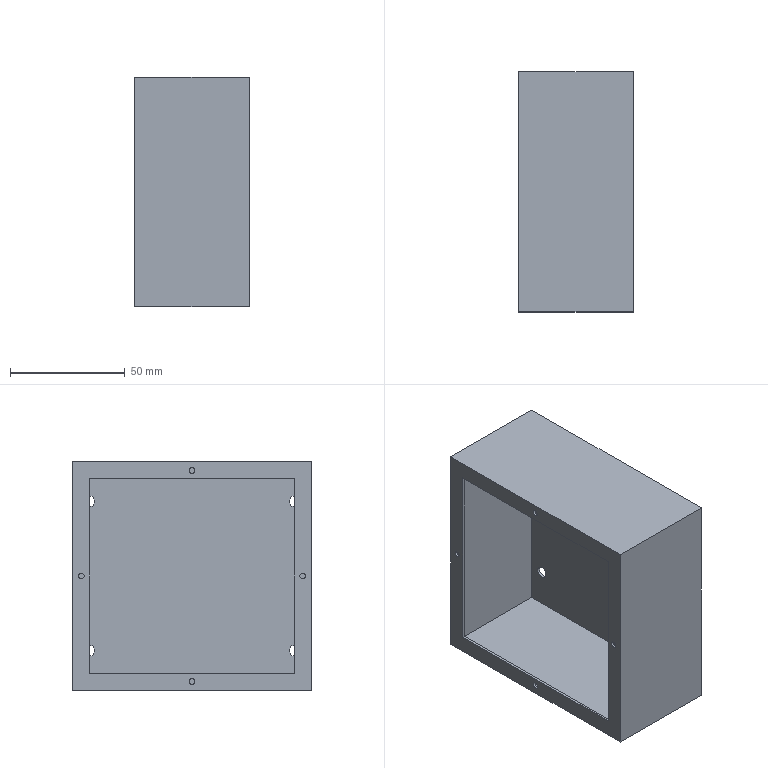Part | STEP file | 2026.6.15-Main Assembly图.sldasm-Part-141 | 1 solid | 32 faces | box 50 x 104.5 x 100 mm | volume 32634 mm3 | cylinder 16 | plane 16 | commonest cylinder face diameters 2.5 x8 5 x8
STEP:
#1=CARTESIAN_POINT('',(-1735.724,608.801,4186.167));
#2=VERTEX_POINT('',#1);
#3=CARTESIAN_POINT('',(-1735.724,606.301,4186.167));
#4=VERTEX_POINT('',#3);
#5=CARTESIAN_POINT('',(-1735.724,607.551,4186.167));
#6=DIRECTION('',(-1.,0.,0.));
#7=DIRECTION('',(0.,0.,1.));
#8=AXIS2_PLACEMENT_3D('',#5,#6,#7);
#9=CIRCLE('',#8,1.25);
#10=EDGE_CURVE('',#2,#4,#9,.T.);
#11=ORIENTED_EDGE('',*,*,#10,.F.);
#12=CARTESIAN_POINT('',(-1736.724,608.801,4186.167));
#13=VERTEX_POINT('',#12);
#14=CARTESIAN_POINT('',(-1735.724,608.801,4186.167));
#15=DIRECTION('',(-1.,0.,0.));
#16=VECTOR('',#15,1000.);
#17=LINE('',#14,#16);
#18=EDGE_CURVE('',#2,#13,#17,.T.);
#19=ORIENTED_EDGE('',*,*,#18,.T.);
#20=CARTESIAN_POINT('',(-1736.724,606.301,4186.167));
#21=VERTEX_POINT('',#20);
#22=CARTESIAN_POINT('',(-1736.724,607.551,4186.167));
#23=DIRECTION('',(-1.,0.,0.));
#24=DIRECTION('',(0.,0.,1.));
#25=AXIS2_PLACEMENT_3D('',#22,#23,#24);
#26=CIRCLE('',#25,1.25);
#27=EDGE_CURVE('',#13,#21,#26,.T.);
#28=ORIENTED_EDGE('',*,*,#27,.T.);
#29=CARTESIAN_POINT('',(-1735.724,606.301,4186.167));
#30=DIRECTION('',(-1.,0.,0.));
#31=VECTOR('',#30,1000.);
#32=LINE('',#29,#31);
#33=EDGE_CURVE('',#4,#21,#32,.T.);
#34=ORIENTED_EDGE('',*,*,#33,.F.);
#35=EDGE_LOOP('',(#11,#19,#28,#34));
#36=FACE_OUTER_BOUND('',#35,.T.);
#37=CARTESIAN_POINT('',(-1735.724,607.551,4186.167));
#38=DIRECTION('',(-1.,0.,0.));
#39=DIRECTION('',(0.,-1.,0.));
#40=AXIS2_PLACEMENT_3D('',#37,#38,#39);
#41=CYLINDRICAL_SURFACE('',#40,1.25);
#42=ADVANCED_FACE('',(#36),#41,.F.);
#43=CARTESIAN_POINT('',(-1735.724,560.551,4140.167));
#44=VERTEX_POINT('',#43);
#45=CARTESIAN_POINT('',(-1735.724,558.051,4140.167));
#46=VERTEX_POINT('',#45);
#47=CARTESIAN_POINT('',(-1735.724,559.301,4140.167));
#48=DIRECTION('',(-1.,0.,0.));
#49=DIRECTION('',(0.,0.,1.));
#50=AXIS2_PLACEMENT_3D('',#47,#48,#49);
#51=CIRCLE('',#50,1.25);
#52=EDGE_CURVE('',#44,#46,#51,.T.);
#53=ORIENTED_EDGE('',*,*,#52,.F.);
#54=CARTESIAN_POINT('',(-1736.724,560.551,4140.167));
#55=VERTEX_POINT('',#54);
#56=CARTESIAN_POINT('',(-1735.724,560.551,4140.167));
#57=DIRECTION('',(-1.,0.,0.));
#58=VECTOR('',#57,1000.);
#59=LINE('',#56,#58);
#60=EDGE_CURVE('',#44,#55,#59,.T.);
#61=ORIENTED_EDGE('',*,*,#60,.T.);
#62=CARTESIAN_POINT('',(-1736.724,558.051,4140.167));
#63=VERTEX_POINT('',#62);
#64=CARTESIAN_POINT('',(-1736.724,559.301,4140.167));
#65=DIRECTION('',(-1.,0.,0.));
#66=DIRECTION('',(0.,0.,1.));
#67=AXIS2_PLACEMENT_3D('',#64,#65,#66);
#68=CIRCLE('',#67,1.25);
#69=EDGE_CURVE('',#55,#63,#68,.T.);
#70=ORIENTED_EDGE('',*,*,#69,.T.);
#71=CARTESIAN_POINT('',(-1735.724,558.051,4140.167));
#72=DIRECTION('',(-1.,0.,0.));
#73=VECTOR('',#72,1000.);
#74=LINE('',#71,#73);
#75=EDGE_CURVE('',#46,#63,#74,.T.);
#76=ORIENTED_EDGE('',*,*,#75,.F.);
#77=EDGE_LOOP('',(#53,#61,#70,#76));
#78=FACE_OUTER_BOUND('',#77,.T.);
#79=CARTESIAN_POINT('',(-1735.724,559.301,4140.167));
#80=DIRECTION('',(-1.,0.,0.));
#81=DIRECTION('',(0.,-1.,0.));
#82=AXIS2_PLACEMENT_3D('',#79,#80,#81);
#83=CYLINDRICAL_SURFACE('',#82,1.25);
#84=ADVANCED_FACE('',(#78),#83,.F.);
#85=CARTESIAN_POINT('',(-1735.724,512.301,4186.167));
#86=VERTEX_POINT('',#85);
#87=CARTESIAN_POINT('',(-1735.724,509.801,4186.167));
#88=VERTEX_POINT('',#87);
#89=CARTESIAN_POINT('',(-1735.724,511.051,4186.167));
#90=DIRECTION('',(-1.,0.,0.));
#91=DIRECTION('',(0.,0.,1.));
#92=AXIS2_PLACEMENT_3D('',#89,#90,#91);
#93=CIRCLE('',#92,1.25);
#94=EDGE_CURVE('',#86,#88,#93,.T.);
#95=ORIENTED_EDGE('',*,*,#94,.F.);
#96=CARTESIAN_POINT('',(-1736.724,512.301,4186.167));
#97=VERTEX_POINT('',#96);
#98=CARTESIAN_POINT('',(-1735.724,512.301,4186.167));
#99=DIRECTION('',(-1.,0.,0.));
#100=VECTOR('',#99,1000.);
#101=LINE('',#98,#100);
#102=EDGE_CURVE('',#86,#97,#101,.T.);
#103=ORIENTED_EDGE('',*,*,#102,.T.);
#104=CARTESIAN_POINT('',(-1736.724,509.801,4186.167));
#105=VERTEX_POINT('',#104);
#106=CARTESIAN_POINT('',(-1736.724,511.051,4186.167));
#107=DIRECTION('',(-1.,0.,0.));
#108=DIRECTION('',(0.,0.,1.));
#109=AXIS2_PLACEMENT_3D('',#106,#107,#108);
#110=CIRCLE('',#109,1.25);
#111=EDGE_CURVE('',#97,#105,#110,.T.);
#112=ORIENTED_EDGE('',*,*,#111,.T.);
#113=CARTESIAN_POINT('',(-1735.724,509.801,4186.167));
#114=DIRECTION('',(-1.,0.,0.));
#115=VECTOR('',#114,1000.);
#116=LINE('',#113,#115);
#117=EDGE_CURVE('',#88,#105,#116,.T.);
#118=ORIENTED_EDGE('',*,*,#117,.F.);
#119=EDGE_LOOP('',(#95,#103,#112,#118));
#120=FACE_OUTER_BOUND('',#119,.T.);
#121=CARTESIAN_POINT('',(-1735.724,511.051,4186.167));
#122=DIRECTION('',(-1.,0.,0.));
#123=DIRECTION('',(0.,-1.,0.));
#124=AXIS2_PLACEMENT_3D('',#121,#122,#123);
#125=CYLINDRICAL_SURFACE('',#124,1.25);
#126=ADVANCED_FACE('',(#120),#125,.F.);
#127=CARTESIAN_POINT('',(-1735.724,560.551,4232.167));
#128=VERTEX_POINT('',#127);
#129=CARTESIAN_POINT('',(-1735.724,558.051,4232.167));
#130=VERTEX_POINT('',#129);
#131=CARTESIAN_POINT('',(-1735.724,559.301,4232.167));
#132=DIRECTION('',(-1.,0.,0.));
#133=DIRECTION('',(0.,0.,1.));
#134=AXIS2_PLACEMENT_3D('',#131,#132,#133);
#135=CIRCLE('',#134,1.25);
#136=EDGE_CURVE('',#128,#130,#135,.T.);
#137=ORIENTED_EDGE('',*,*,#136,.F.);
#138=CARTESIAN_POINT('',(-1736.724,560.551,4232.167));
#139=VERTEX_POINT('',#138);
#140=CARTESIAN_POINT('',(-1735.724,560.551,4232.167));
#141=DIRECTION('',(-1.,0.,0.));
#142=VECTOR('',#141,1000.);
#143=LINE('',#140,#142);
#144=EDGE_CURVE('',#128,#139,#143,.T.);
#145=ORIENTED_EDGE('',*,*,#144,.T.);
#146=CARTESIAN_POINT('',(-1736.724,558.051,4232.167));
#147=VERTEX_POINT('',#146);
#148=CARTESIAN_POINT('',(-1736.724,559.301,4232.167));
#149=DIRECTION('',(-1.,0.,0.));
#150=DIRECTION('',(0.,0.,1.));
#151=AXIS2_PLACEMENT_3D('',#148,#149,#150);
#152=CIRCLE('',#151,1.25);
#153=EDGE_CURVE('',#139,#147,#152,.T.);
#154=ORIENTED_EDGE('',*,*,#153,.T.);
#155=CARTESIAN_POINT('',(-1735.724,558.051,4232.167));
#156=DIRECTION('',(-1.,0.,0.));
#157=VECTOR('',#156,1000.);
#158=LINE('',#155,#157);
#159=EDGE_CURVE('',#130,#147,#158,.T.);
#160=ORIENTED_EDGE('',*,*,#159,.F.);
#161=EDGE_LOOP('',(#137,#145,#154,#160));
#162=FACE_OUTER_BOUND('',#161,.T.);
#163=CARTESIAN_POINT('',(-1735.724,559.301,4232.167));
#164=DIRECTION('',(-1.,0.,0.));
#165=DIRECTION('',(0.,-1.,0.));
#166=AXIS2_PLACEMENT_3D('',#163,#164,#165);
#167=CYLINDRICAL_SURFACE('',#166,1.25);
#168=ADVANCED_FACE('',(#162),#167,.F.);
#169=CARTESIAN_POINT('',(-1687.724,511.801,4153.667));
#170=VERTEX_POINT('',#169);
#171=CARTESIAN_POINT('',(-1687.724,516.801,4153.667));
#172=VERTEX_POINT('',#171);
#173=CARTESIAN_POINT('',(-1687.724,514.301,4153.667));
#174=DIRECTION('',(1.,0.,0.));
#175=DIRECTION('',(0.,0.,-1.));
#176=AXIS2_PLACEMENT_3D('',#173,#174,#175);
#177=CIRCLE('',#176,2.5);
#178=EDGE_CURVE('',#170,#172,#177,.T.);
#179=ORIENTED_EDGE('',*,*,#178,.F.);
#180=CARTESIAN_POINT('',(-1686.724,511.801,4153.667));
#181=VERTEX_POINT('',#180);
#182=CARTESIAN_POINT('',(-1687.724,511.801,4153.667));
#183=DIRECTION('',(1.,0.,0.));
#184=VECTOR('',#183,1000.);
#185=LINE('',#182,#184);
#186=EDGE_CURVE('',#170,#181,#185,.T.);
#187=ORIENTED_EDGE('',*,*,#186,.T.);
#188=CARTESIAN_POINT('',(-1686.724,516.801,4153.667));
#189=VERTEX_POINT('',#188);
#190=CARTESIAN_POINT('',(-1686.724,514.301,4153.667));
#191=DIRECTION('',(1.,0.,0.));
#192=DIRECTION('',(0.,0.,-1.));
#193=AXIS2_PLACEMENT_3D('',#190,#191,#192);
#194=CIRCLE('',#193,2.5);
#195=EDGE_CURVE('',#181,#189,#194,.T.);
#196=ORIENTED_EDGE('',*,*,#195,.T.);
#197=CARTESIAN_POINT('',(-1687.724,516.801,4153.667));
#198=DIRECTION('',(1.,0.,0.));
#199=VECTOR('',#198,1000.);
#200=LINE('',#197,#199);
#201=EDGE_CURVE('',#172,#189,#200,.T.);
#202=ORIENTED_EDGE('',*,*,#201,.F.);
#203=EDGE_LOOP('',(#179,#187,#196,#202));
#204=FACE_OUTER_BOUND('',#203,.T.);
#205=CARTESIAN_POINT('',(-1687.724,514.301,4153.667));
#206=DIRECTION('',(1.,0.,0.));
#207=DIRECTION('',(0.,1.,0.));
#208=AXIS2_PLACEMENT_3D('',#205,#206,#207);
#209=CYLINDRICAL_SURFACE('',#208,2.5);
#210=ADVANCED_FACE('',(#204),#209,.F.);
#211=CARTESIAN_POINT('',(-1687.724,601.801,4218.667));
#212=VERTEX_POINT('',#211);
#213=CARTESIAN_POINT('',(-1687.724,606.801,4218.667));
#214=VERTEX_POINT('',#213);
#215=CARTESIAN_POINT('',(-1687.724,604.301,4218.667));
#216=DIRECTION('',(1.,0.,0.));
#217=DIRECTION('',(0.,0.,-1.));
#218=AXIS2_PLACEMENT_3D('',#215,#216,#217);
#219=CIRCLE('',#218,2.5);
#220=EDGE_CURVE('',#212,#214,#219,.T.);
#221=ORIENTED_EDGE('',*,*,#220,.F.);
#222=CARTESIAN_POINT('',(-1686.724,601.801,4218.667));
#223=VERTEX_POINT('',#222);
#224=CARTESIAN_POINT('',(-1687.724,601.801,4218.667));
#225=DIRECTION('',(1.,0.,0.));
#226=VECTOR('',#225,1000.);
#227=LINE('',#224,#226);
#228=EDGE_CURVE('',#212,#223,#227,.T.);
#229=ORIENTED_EDGE('',*,*,#228,.T.);
#230=CARTESIAN_POINT('',(-1686.724,606.801,4218.667));
#231=VERTEX_POINT('',#230);
#232=CARTESIAN_POINT('',(-1686.724,604.301,4218.667));
#233=DIRECTION('',(1.,0.,0.));
#234=DIRECTION('',(0.,0.,-1.));
#235=AXIS2_PLACEMENT_3D('',#232,#233,#234);
#236=CIRCLE('',#235,2.5);
#237=EDGE_CURVE('',#223,#231,#236,.T.);
#238=ORIENTED_EDGE('',*,*,#237,.T.);
#239=CARTESIAN_POINT('',(-1687.724,606.801,4218.667));
#240=DIRECTION('',(1.,0.,0.));
#241=VECTOR('',#240,1000.);
#242=LINE('',#239,#241);
#243=EDGE_CURVE('',#214,#231,#242,.T.);
#244=ORIENTED_EDGE('',*,*,#243,.F.);
#245=EDGE_LOOP('',(#221,#229,#238,#244));
#246=FACE_OUTER_BOUND('',#245,.T.);
#247=CARTESIAN_POINT('',(-1687.724,604.301,4218.667));
#248=DIRECTION('',(1.,0.,0.));
#249=DIRECTION('',(0.,1.,0.));
#250=AXIS2_PLACEMENT_3D('',#247,#248,#249);
#251=CYLINDRICAL_SURFACE('',#250,2.5);
#252=ADVANCED_FACE('',(#246),#251,.F.);
#253=CARTESIAN_POINT('',(-1687.724,511.801,4218.667));
#254=VERTEX_POINT('',#253);
#255=CARTESIAN_POINT('',(-1687.724,516.801,4218.667));
#256=VERTEX_POINT('',#255);
#257=CARTESIAN_POINT('',(-1687.724,514.301,4218.667));
#258=DIRECTION('',(1.,0.,0.));
#259=DIRECTION('',(0.,0.,-1.));
#260=AXIS2_PLACEMENT_3D('',#257,#258,#259);
#261=CIRCLE('',#260,2.5);
#262=EDGE_CURVE('',#254,#256,#261,.T.);
#263=ORIENTED_EDGE('',*,*,#262,.F.);
#264=CARTESIAN_POINT('',(-1686.724,511.801,4218.667));
#265=VERTEX_POINT('',#264);
#266=CARTESIAN_POINT('',(-1687.724,511.801,4218.667));
#267=DIRECTION('',(1.,0.,0.));
#268=VECTOR('',#267,1000.);
#269=LINE('',#266,#268);
#270=EDGE_CURVE('',#254,#265,#269,.T.);
#271=ORIENTED_EDGE('',*,*,#270,.T.);
#272=CARTESIAN_POINT('',(-1686.724,516.801,4218.667));
#273=VERTEX_POINT('',#272);
#274=CARTESIAN_POINT('',(-1686.724,514.301,4218.667));
#275=DIRECTION('',(1.,0.,0.));
#276=DIRECTION('',(0.,0.,-1.));
#277=AXIS2_PLACEMENT_3D('',#274,#275,#276);
#278=CIRCLE('',#277,2.5);
#279=EDGE_CURVE('',#265,#273,#278,.T.);
#280=ORIENTED_EDGE('',*,*,#279,.T.);
#281=CARTESIAN_POINT('',(-1687.724,516.801,4218.667));
#282=DIRECTION('',(1.,0.,0.));
#283=VECTOR('',#282,1000.);
#284=LINE('',#281,#283);
#285=EDGE_CURVE('',#256,#273,#284,.T.);
#286=ORIENTED_EDGE('',*,*,#285,.F.);
#287=EDGE_LOOP('',(#263,#271,#280,#286));
#288=FACE_OUTER_BOUND('',#287,.T.);
#289=CARTESIAN_POINT('',(-1687.724,514.301,4218.667));
#290=DIRECTION('',(1.,0.,0.));
#291=DIRECTION('',(0.,1.,0.));
#292=AXIS2_PLACEMENT_3D('',#289,#290,#291);
#293=CYLINDRICAL_SURFACE('',#292,2.5);
#294=ADVANCED_FACE('',(#288),#293,.F.);
#295=CARTESIAN_POINT('',(-1687.724,601.801,4153.667));
#296=VERTEX_POINT('',#295);
#297=CARTESIAN_POINT('',(-1687.724,606.801,4153.667));
#298=VERTEX_POINT('',#297);
#299=CARTESIAN_POINT('',(-1687.724,604.301,4153.667));
#300=DIRECTION('',(1.,0.,0.));
#301=DIRECTION('',(0.,0.,-1.));
#302=AXIS2_PLACEMENT_3D('',#299,#300,#301);
#303=CIRCLE('',#302,2.5);
#304=EDGE_CURVE('',#296,#298,#303,.T.);
#305=ORIENTED_EDGE('',*,*,#304,.F.);
#306=CARTESIAN_POINT('',(-1686.724,601.801,4153.667));
#307=VERTEX_POINT('',#306);
#308=CARTESIAN_POINT('',(-1687.724,601.801,4153.667));
#309=DIRECTION('',(1.,0.,0.));
#310=VECTOR('',#309,1000.);
#311=LINE('',#308,#310);
#312=EDGE_CURVE('',#296,#307,#311,.T.);
#313=ORIENTED_EDGE('',*,*,#312,.T.);
#314=CARTESIAN_POINT('',(-1686.724,606.801,4153.667));
#315=VERTEX_POINT('',#314);
#316=CARTESIAN_POINT('',(-1686.724,604.301,4153.667));
#317=DIRECTION('',(1.,0.,0.));
#318=DIRECTION('',(0.,0.,-1.));
#319=AXIS2_PLACEMENT_3D('',#316,#317,#318);
#320=CIRCLE('',#319,2.5);
#321=EDGE_CURVE('',#307,#315,#320,.T.);
#322=ORIENTED_EDGE('',*,*,#321,.T.);
#323=CARTESIAN_POINT('',(-1687.724,606.801,4153.667));
#324=DIRECTION('',(1.,0.,0.));
#325=VECTOR('',#324,1000.);
#326=LINE('',#323,#325);
#327=EDGE_CURVE('',#298,#315,#326,.T.);
#328=ORIENTED_EDGE('',*,*,#327,.F.);
#329=EDGE_LOOP('',(#305,#313,#322,#328));
#330=FACE_OUTER_BOUND('',#329,.T.);
#331=CARTESIAN_POINT('',(-1687.724,604.301,4153.667));
#332=DIRECTION('',(1.,0.,0.));
#333=DIRECTION('',(0.,1.,0.));
#334=AXIS2_PLACEMENT_3D('',#331,#332,#333);
#335=CYLINDRICAL_SURFACE('',#334,2.5);
#336=ADVANCED_FACE('',(#330),#335,.F.);
#337=CARTESIAN_POINT('',(-1686.724,611.551,4136.167));
#338=VERTEX_POINT('',#337);
#339=CARTESIAN_POINT('',(-1686.724,507.051,4136.167));
#340=VERTEX_POINT('',#339);
#341=CARTESIAN_POINT('',(-1686.724,611.551,4136.167));
#342=DIRECTION('',(0.,-1.,0.));
#343=VECTOR('',#342,1000.);
#344=LINE('',#341,#343);
#345=EDGE_CURVE('',#338,#340,#344,.T.);
#346=ORIENTED_EDGE('',*,*,#345,.T.);
#347=CARTESIAN_POINT('',(-1736.724,507.051,4136.167));
#348=VERTEX_POINT('',#347);
#349=CARTESIAN_POINT('',(-1687.724,507.051,4136.167));
#350=DIRECTION('',(1.,0.,0.));
#351=VECTOR('',#350,1000.);
#352=LINE('',#349,#351);
#353=EDGE_CURVE('',#348,#340,#352,.T.);
#354=ORIENTED_EDGE('',*,*,#353,.F.);
#355=CARTESIAN_POINT('',(-1736.724,611.551,4136.167));
#356=VERTEX_POINT('',#355);
#357=CARTESIAN_POINT('',(-1736.724,611.551,4136.167));
#358=DIRECTION('',(0.,-1.,0.));
#359=VECTOR('',#358,1000.);
#360=LINE('',#357,#359);
#361=EDGE_CURVE('',#356,#348,#360,.T.);
#362=ORIENTED_EDGE('',*,*,#361,.F.);
#363=CARTESIAN_POINT('',(-1687.724,611.551,4136.167));
#364=DIRECTION('',(1.,0.,0.));
#365=VECTOR('',#364,1000.);
#366=LINE('',#363,#365);
#367=EDGE_CURVE('',#356,#338,#366,.T.);
#368=ORIENTED_EDGE('',*,*,#367,.T.);
#369=EDGE_LOOP('',(#346,#354,#362,#368));
#370=FACE_OUTER_BOUND('',#369,.T.);
#371=CARTESIAN_POINT('',(-1687.724,611.551,4136.167));
#372=DIRECTION('',(0.,0.,1.));
#373=DIRECTION('',(1.,0.,0.));
#374=AXIS2_PLACEMENT_3D('',#371,#372,#373);
#375=PLANE('',#374);
#376=ADVANCED_FACE('',(#370),#375,.F.);
#377=CARTESIAN_POINT('',(-1686.724,507.051,4236.167));
#378=VERTEX_POINT('',#377);
#379=CARTESIAN_POINT('',(-1686.724,507.051,4136.167));
#380=DIRECTION('',(0.,0.,1.));
#381=VECTOR('',#380,1000.);
#382=LINE('',#379,#381);
#383=EDGE_CURVE('',#340,#378,#382,.T.);
#384=ORIENTED_EDGE('',*,*,#383,.T.);
#385=CARTESIAN_POINT('',(-1736.724,507.051,4236.167));
#386=VERTEX_POINT('',#385);
#387=CARTESIAN_POINT('',(-1687.724,507.051,4236.167));
#388=DIRECTION('',(1.,0.,0.));
#389=VECTOR('',#388,1000.);
#390=LINE('',#387,#389);
#391=EDGE_CURVE('',#386,#378,#390,.T.);
#392=ORIENTED_EDGE('',*,*,#391,.F.);
#393=CARTESIAN_POINT('',(-1736.724,507.051,4136.167));
#394=DIRECTION('',(0.,0.,1.));
#395=VECTOR('',#394,1000.);
#396=LINE('',#393,#395);
#397=EDGE_CURVE('',#348,#386,#396,.T.);
#398=ORIENTED_EDGE('',*,*,#397,.F.);
#399=ORIENTED_EDGE('',*,*,#353,.T.);
#400=EDGE_LOOP('',(#384,#392,#398,#399));
#401=FACE_OUTER_BOUND('',#400,.T.);
#402=CARTESIAN_POINT('',(-1687.724,507.051,4136.167));
#403=DIRECTION('',(0.,1.,0.));
#404=DIRECTION('',(0.,0.,1.));
#405=AXIS2_PLACEMENT_3D('',#402,#403,#404);
#406=PLANE('',#405);
#407=ADVANCED_FACE('',(#401),#406,.F.);
#408=CARTESIAN_POINT('',(-1686.724,611.551,4236.167));
#409=VERTEX_POINT('',#408);
#410=CARTESIAN_POINT('',(-1686.724,507.051,4236.167));
#411=DIRECTION('',(0.,1.,0.));
#412=VECTOR('',#411,1000.);
#413=LINE('',#410,#412);
#414=EDGE_CURVE('',#378,#409,#413,.T.);
#415=ORIENTED_EDGE('',*,*,#414,.T.);
#416=CARTESIAN_POINT('',(-1736.724,611.551,4236.167));
#417=VERTEX_POINT('',#416);
#418=CARTESIAN_POINT('',(-1687.724,611.551,4236.167));
#419=DIRECTION('',(1.,0.,0.));
#420=VECTOR('',#419,1000.);
#421=LINE('',#418,#420);
#422=EDGE_CURVE('',#417,#409,#421,.T.);
#423=ORIENTED_EDGE('',*,*,#422,.F.);
#424=CARTESIAN_POINT('',(-1736.724,507.051,4236.167));
#425=DIRECTION('',(0.,1.,0.));
#426=VECTOR('',#425,1000.);
#427=LINE('',#424,#426);
#428=EDGE_CURVE('',#386,#417,#427,.T.);
#429=ORIENTED_EDGE('',*,*,#428,.F.);
#430=ORIENTED_EDGE('',*,*,#391,.T.);
#431=EDGE_LOOP('',(#415,#423,#429,#430));
#432=FACE_OUTER_BOUND('',#431,.T.);
#433=CARTESIAN_POINT('',(-1687.724,507.051,4236.167));
#434=DIRECTION('',(0.,0.,-1.));
#435=DIRECTION('',(-1.,0.,0.));
#436=AXIS2_PLACEMENT_3D('',#433,#434,#435);
#437=PLANE('',#436);
#438=ADVANCED_FACE('',(#432),#437,.F.);
#439=ORIENTED_EDGE('',*,*,#312,.F.);
#440=CARTESIAN_POINT('',(-1687.724,604.301,4153.667));
#441=DIRECTION('',(1.,0.,0.));
#442=DIRECTION('',(0.,0.,-1.));
#443=AXIS2_PLACEMENT_3D('',#440,#441,#442);
#444=CIRCLE('',#443,2.5);
#445=EDGE_CURVE('',#298,#296,#444,.T.);
#446=ORIENTED_EDGE('',*,*,#445,.F.);
#447=ORIENTED_EDGE('',*,*,#327,.T.);
#448=CARTESIAN_POINT('',(-1686.724,604.301,4153.667));
#449=DIRECTION('',(1.,0.,0.));
#450=DIRECTION('',(0.,0.,-1.));
#451=AXIS2_PLACEMENT_3D('',#448,#449,#450);
#452=CIRCLE('',#451,2.5);
#453=EDGE_CURVE('',#315,#307,#452,.T.);
#454=ORIENTED_EDGE('',*,*,#453,.T.);
#455=EDGE_LOOP('',(#439,#446,#447,#454));
#456=FACE_OUTER_BOUND('',#455,.T.);
#457=CARTESIAN_POINT('',(-1687.724,604.301,4153.667));
#458=DIRECTION('',(1.,0.,0.));
#459=DIRECTION('',(0.,1.,0.));
#460=AXIS2_PLACEMENT_3D('',#457,#458,#459);
#461=CYLINDRICAL_SURFACE('',#460,2.5);
#462=ADVANCED_FACE('',(#456),#461,.F.);
#463=ORIENTED_EDGE('',*,*,#270,.F.);
#464=CARTESIAN_POINT('',(-1687.724,514.301,4218.667));
#465=DIRECTION('',(1.,0.,0.));
#466=DIRECTION('',(0.,0.,-1.));
#467=AXIS2_PLACEMENT_3D('',#464,#465,#466);
#468=CIRCLE('',#467,2.5);
#469=EDGE_CURVE('',#256,#254,#468,.T.);
#470=ORIENTED_EDGE('',*,*,#469,.F.);
#471=ORIENTED_EDGE('',*,*,#285,.T.);
#472=CARTESIAN_POINT('',(-1686.724,514.301,4218.667));
#473=DIRECTION('',(1.,0.,0.));
#474=DIRECTION('',(0.,0.,-1.));
#475=AXIS2_PLACEMENT_3D('',#472,#473,#474);
#476=CIRCLE('',#475,2.5);
#477=EDGE_CURVE('',#273,#265,#476,.T.);
#478=ORIENTED_EDGE('',*,*,#477,.T.);
#479=EDGE_LOOP('',(#463,#470,#471,#478));
#480=FACE_OUTER_BOUND('',#479,.T.);
#481=CARTESIAN_POINT('',(-1687.724,514.301,4218.667));
#482=DIRECTION('',(1.,0.,0.));
#483=DIRECTION('',(0.,1.,0.));
#484=AXIS2_PLACEMENT_3D('',#481,#482,#483);
#485=CYLINDRICAL_SURFACE('',#484,2.5);
#486=ADVANCED_FACE('',(#480),#485,.F.);
#487=ORIENTED_EDGE('',*,*,#228,.F.);
#488=CARTESIAN_POINT('',(-1687.724,604.301,4218.667));
#489=DIRECTION('',(1.,0.,0.));
#490=DIRECTION('',(0.,0.,-1.));
#491=AXIS2_PLACEMENT_3D('',#488,#489,#490);
#492=CIRCLE('',#491,2.5);
#493=EDGE_CURVE('',#214,#212,#492,.T.);
#494=ORIENTED_EDGE('',*,*,#493,.F.);
#495=ORIENTED_EDGE('',*,*,#243,.T.);
#496=CARTESIAN_POINT('',(-1686.724,604.301,4218.667));
#497=DIRECTION('',(1.,0.,0.));
#498=DIRECTION('',(0.,0.,-1.));
#499=AXIS2_PLACEMENT_3D('',#496,#497,#498);
#500=CIRCLE('',#499,2.5);
#501=EDGE_CURVE('',#231,#223,#500,.T.);
#502=ORIENTED_EDGE('',*,*,#501,.T.);
#503=EDGE_LOOP('',(#487,#494,#495,#502));
#504=FACE_OUTER_BOUND('',#503,.T.);
#505=CARTESIAN_POINT('',(-1687.724,604.301,4218.667));
#506=DIRECTION('',(1.,0.,0.));
#507=DIRECTION('',(0.,1.,0.));
#508=AXIS2_PLACEMENT_3D('',#505,#506,#507);
#509=CYLINDRICAL_SURFACE('',#508,2.5);
#510=ADVANCED_FACE('',(#504),#509,.F.);
#511=CARTESIAN_POINT('',(-1686.724,611.551,4236.167));
#512=DIRECTION('',(0.,0.,-1.));
#513=VECTOR('',#512,1000.);
#514=LINE('',#511,#513);
#515=EDGE_CURVE('',#409,#338,#514,.T.);
#516=ORIENTED_EDGE('',*,*,#515,.T.);
#517=ORIENTED_EDGE('',*,*,#367,.F.);
#518=CARTESIAN_POINT('',(-1736.724,611.551,4236.167));
#519=DIRECTION('',(0.,0.,-1.));
#520=VECTOR('',#519,1000.);
#521=LINE('',#518,#520);
#522=EDGE_CURVE('',#417,#356,#521,.T.);
#523=ORIENTED_EDGE('',*,*,#522,.F.);
#524=ORIENTED_EDGE('',*,*,#422,.T.);
#525=EDGE_LOOP('',(#516,#517,#523,#524));
#526=FACE_OUTER_BOUND('',#525,.T.);
#527=CARTESIAN_POINT('',(-1687.724,611.551,4236.167));
#528=DIRECTION('',(0.,-1.,0.));
#529=DIRECTION('',(1.,0.,0.));
#530=AXIS2_PLACEMENT_3D('',#527,#528,#529);
#531=PLANE('',#530);
#532=ADVANCED_FACE('',(#526),#531,.F.);
#533=ORIENTED_EDGE('',*,*,#186,.F.);
#534=CARTESIAN_POINT('',(-1687.724,514.301,4153.667));
#535=DIRECTION('',(1.,0.,0.));
#536=DIRECTION('',(0.,0.,-1.));
#537=AXIS2_PLACEMENT_3D('',#534,#535,#536);
#538=CIRCLE('',#537,2.5);
#539=EDGE_CURVE('',#172,#170,#538,.T.);
#540=ORIENTED_EDGE('',*,*,#539,.F.);
#541=ORIENTED_EDGE('',*,*,#201,.T.);
#542=CARTESIAN_POINT('',(-1686.724,514.301,4153.667));
#543=DIRECTION('',(1.,0.,0.));
#544=DIRECTION('',(0.,0.,-1.));
#545=AXIS2_PLACEMENT_3D('',#542,#543,#544);
#546=CIRCLE('',#545,2.5);
#547=EDGE_CURVE('',#189,#181,#546,.T.);
#548=ORIENTED_EDGE('',*,*,#547,.T.);
#549=EDGE_LOOP('',(#533,#540,#541,#548));
#550=FACE_OUTER_BOUND('',#549,.T.);
#551=CARTESIAN_POINT('',(-1687.724,514.301,4153.667));
#552=DIRECTION('',(1.,0.,0.));
#553=DIRECTION('',(0.,1.,0.));
#554=AXIS2_PLACEMENT_3D('',#551,#552,#553);
#555=CYLINDRICAL_SURFACE('',#554,2.5);
#556=ADVANCED_FACE('',(#550),#555,.F.);
#557=CARTESIAN_POINT('',(-1687.724,610.551,4137.167));
#558=VERTEX_POINT('',#557);
#559=CARTESIAN_POINT('',(-1687.724,508.051,4137.167));
#560=VERTEX_POINT('',#559);
#561=CARTESIAN_POINT('',(-1687.724,611.551,4137.167));
#562=DIRECTION('',(0.,-1.,0.));
#563=VECTOR('',#562,1000.);
#564=LINE('',#561,#563);
#565=EDGE_CURVE('',#558,#560,#564,.T.);
#566=ORIENTED_EDGE('',*,*,#565,.T.);
#567=CARTESIAN_POINT('',(-1687.724,508.051,4235.167));
#568=VERTEX_POINT('',#567);
#569=CARTESIAN_POINT('',(-1687.724,508.051,4136.167));
#570=DIRECTION('',(0.,0.,1.));
#571=VECTOR('',#570,1000.);
#572=LINE('',#569,#571);
#573=EDGE_CURVE('',#560,#568,#572,.T.);
#574=ORIENTED_EDGE('',*,*,#573,.T.);
#575=CARTESIAN_POINT('',(-1687.724,610.551,4235.167));
#576=VERTEX_POINT('',#575);
#577=CARTESIAN_POINT('',(-1687.724,507.051,4235.167));
#578=DIRECTION('',(0.,1.,0.));
#579=VECTOR('',#578,1000.);
#580=LINE('',#577,#579);
#581=EDGE_CURVE('',#568,#576,#580,.T.);
#582=ORIENTED_EDGE('',*,*,#581,.T.);
#583=CARTESIAN_POINT('',(-1687.724,610.551,4236.167));
#584=DIRECTION('',(0.,0.,-1.));
#585=VECTOR('',#584,1000.);
#586=LINE('',#583,#585);
#587=EDGE_CURVE('',#576,#558,#586,.T.);
#588=ORIENTED_EDGE('',*,*,#587,.T.);
#589=EDGE_LOOP('',(#566,#574,#582,#588));
#590=FACE_OUTER_BOUND('',#589,.T.);
#591=ORIENTED_EDGE('',*,*,#493,.T.);
#592=ORIENTED_EDGE('',*,*,#220,.T.);
#593=EDGE_LOOP('',(#591,#592));
#594=FACE_BOUND('',#593,.T.);
#595=ORIENTED_EDGE('',*,*,#469,.T.);
#596=ORIENTED_EDGE('',*,*,#262,.T.);
#597=EDGE_LOOP('',(#595,#596));
#598=FACE_BOUND('',#597,.T.);
#599=ORIENTED_EDGE('',*,*,#445,.T.);
#600=ORIENTED_EDGE('',*,*,#304,.T.);
#601=EDGE_LOOP('',(#599,#600));
#602=FACE_BOUND('',#601,.T.);
#603=ORIENTED_EDGE('',*,*,#539,.T.);
#604=ORIENTED_EDGE('',*,*,#178,.T.);
#605=EDGE_LOOP('',(#603,#604));
#606=FACE_BOUND('',#605,.T.);
#607=CARTESIAN_POINT('',(-1687.724,604.301,4218.667));
#608=DIRECTION('',(1.,0.,0.));
#609=DIRECTION('',(0.,1.,0.));
#610=AXIS2_PLACEMENT_3D('',#607,#608,#609);
#611=PLANE('',#610);
#612=ADVANCED_FACE('',(#590,#594,#598,#602,#606),#611,.F.);
#613=ORIENTED_EDGE('',*,*,#345,.F.);
#614=ORIENTED_EDGE('',*,*,#515,.F.);
#615=ORIENTED_EDGE('',*,*,#414,.F.);
#616=ORIENTED_EDGE('',*,*,#383,.F.);
#617=EDGE_LOOP('',(#613,#614,#615,#616));
#618=FACE_OUTER_BOUND('',#617,.T.);
#619=ORIENTED_EDGE('',*,*,#501,.F.);
#620=ORIENTED_EDGE('',*,*,#237,.F.);
#621=EDGE_LOOP('',(#619,#620));
#622=FACE_BOUND('',#621,.T.);
#623=ORIENTED_EDGE('',*,*,#477,.F.);
#624=ORIENTED_EDGE('',*,*,#279,.F.);
#625=EDGE_LOOP('',(#623,#624));
#626=FACE_BOUND('',#625,.T.);
#627=ORIENTED_EDGE('',*,*,#453,.F.);
#628=ORIENTED_EDGE('',*,*,#321,.F.);
#629=EDGE_LOOP('',(#627,#628));
#630=FACE_BOUND('',#629,.T.);
#631=ORIENTED_EDGE('',*,*,#547,.F.);
#632=ORIENTED_EDGE('',*,*,#195,.F.);
#633=EDGE_LOOP('',(#631,#632));
#634=FACE_BOUND('',#633,.T.);
#635=CARTESIAN_POINT('',(-1686.724,604.301,4218.667));
#636=DIRECTION('',(1.,0.,0.));
#637=DIRECTION('',(0.,1.,0.));
#638=AXIS2_PLACEMENT_3D('',#635,#636,#637);
#639=PLANE('',#638);
#640=ADVANCED_FACE('',(#618,#622,#626,#630,#634),#639,.T.);
#641=CARTESIAN_POINT('',(-1735.724,508.051,4137.167));
#642=VERTEX_POINT('',#641);
#643=CARTESIAN_POINT('',(-1735.724,508.051,4235.167));
#644=VERTEX_POINT('',#643);
#645=CARTESIAN_POINT('',(-1735.724,508.051,4136.167));
#646=DIRECTION('',(0.,0.,1.));
#647=VECTOR('',#646,1000.);
#648=LINE('',#645,#647);
#649=EDGE_CURVE('',#642,#644,#648,.T.);
#650=ORIENTED_EDGE('',*,*,#649,.T.);
#651=CARTESIAN_POINT('',(-1687.724,508.051,4235.167));
#652=DIRECTION('',(-1.,0.,0.));
#653=VECTOR('',#652,1000.);
#654=LINE('',#651,#653);
#655=EDGE_CURVE('',#568,#644,#654,.T.);
#656=ORIENTED_EDGE('',*,*,#655,.F.);
#657=ORIENTED_EDGE('',*,*,#573,.F.);
#658=CARTESIAN_POINT('',(-1687.724,508.051,4137.167));
#659=DIRECTION('',(-1.,0.,0.));
#660=VECTOR('',#659,1000.);
#661=LINE('',#658,#660);
#662=EDGE_CURVE('',#560,#642,#661,.T.);
#663=ORIENTED_EDGE('',*,*,#662,.T.);
#664=EDGE_LOOP('',(#650,#656,#657,#663));
#665=FACE_OUTER_BOUND('',#664,.T.);
#666=CARTESIAN_POINT('',(-1687.724,508.051,4136.167));
#667=DIRECTION('',(0.,-1.,0.));
#668=DIRECTION('',(0.,0.,-1.));
#669=AXIS2_PLACEMENT_3D('',#666,#667,#668);
#670=PLANE('',#669);
#671=ADVANCED_FACE('',(#665),#670,.F.);
#672=CARTESIAN_POINT('',(-1735.724,610.551,4235.167));
#673=VERTEX_POINT('',#672);
#674=CARTESIAN_POINT('',(-1735.724,507.051,4235.167));
#675=DIRECTION('',(0.,1.,0.));
#676=VECTOR('',#675,1000.);
#677=LINE('',#674,#676);
#678=EDGE_CURVE('',#644,#673,#677,.T.);
#679=ORIENTED_EDGE('',*,*,#678,.T.);
#680=CARTESIAN_POINT('',(-1687.724,610.551,4235.167));
#681=DIRECTION('',(-1.,0.,0.));
#682=VECTOR('',#681,1000.);
#683=LINE('',#680,#682);
#684=EDGE_CURVE('',#576,#673,#683,.T.);
#685=ORIENTED_EDGE('',*,*,#684,.F.);
#686=ORIENTED_EDGE('',*,*,#581,.F.);
#687=ORIENTED_EDGE('',*,*,#655,.T.);
#688=EDGE_LOOP('',(#679,#685,#686,#687));
#689=FACE_OUTER_BOUND('',#688,.T.);
#690=CARTESIAN_POINT('',(-1687.724,507.051,4235.167));
#691=DIRECTION('',(0.,0.,1.));
#692=DIRECTION('',(0.,-1.,0.));
#693=AXIS2_PLACEMENT_3D('',#690,#691,#692);
#694=PLANE('',#693);
#695=ADVANCED_FACE('',(#689),#694,.F.);
#696=CARTESIAN_POINT('',(-1735.724,610.551,4137.167));
#697=VERTEX_POINT('',#696);
#698=CARTESIAN_POINT('',(-1735.724,610.551,4236.167));
#699=DIRECTION('',(0.,0.,-1.));
#700=VECTOR('',#699,1000.);
#701=LINE('',#698,#700);
#702=EDGE_CURVE('',#673,#697,#701,.T.);
#703=ORIENTED_EDGE('',*,*,#702,.T.);
#704=CARTESIAN_POINT('',(-1687.724,610.551,4137.167));
#705=DIRECTION('',(-1.,0.,0.));
#706=VECTOR('',#705,1000.);
#707=LINE('',#704,#706);
#708=EDGE_CURVE('',#558,#697,#707,.T.);
#709=ORIENTED_EDGE('',*,*,#708,.F.);
#710=ORIENTED_EDGE('',*,*,#587,.F.);
#711=ORIENTED_EDGE('',*,*,#684,.T.);
#712=EDGE_LOOP('',(#703,#709,#710,#711));
#713=FACE_OUTER_BOUND('',#712,.T.);
#714=CARTESIAN_POINT('',(-1687.724,610.551,4236.167));
#715=DIRECTION('',(0.,1.,0.));
#716=DIRECTION('',(0.,0.,1.));
#717=AXIS2_PLACEMENT_3D('',#714,#715,#716);
#718=PLANE('',#717);
#719=ADVANCED_FACE('',(#713),#718,.F.);
#720=CARTESIAN_POINT('',(-1735.724,611.551,4137.167));
#721=DIRECTION('',(0.,-1.,0.));
#722=VECTOR('',#721,1000.);
#723=LINE('',#720,#722);
#724=EDGE_CURVE('',#697,#642,#723,.T.);
#725=ORIENTED_EDGE('',*,*,#724,.T.);
#726=ORIENTED_EDGE('',*,*,#662,.F.);
#727=ORIENTED_EDGE('',*,*,#565,.F.);
#728=ORIENTED_EDGE('',*,*,#708,.T.);
#729=EDGE_LOOP('',(#725,#726,#727,#728));
#730=FACE_OUTER_BOUND('',#729,.T.);
#731=CARTESIAN_POINT('',(-1687.724,611.551,4137.167));
#732=DIRECTION('',(0.,0.,-1.));
#733=DIRECTION('',(0.,1.,0.));
#734=AXIS2_PLACEMENT_3D('',#731,#732,#733);
#735=PLANE('',#734);
#736=ADVANCED_FACE('',(#730),#735,.F.);
#737=CARTESIAN_POINT('',(-1736.724,604.051,4143.667));
#738=VERTEX_POINT('',#737);
#739=CARTESIAN_POINT('',(-1736.724,514.551,4143.667));
#740=VERTEX_POINT('',#739);
#741=CARTESIAN_POINT('',(-1736.724,604.051,4143.667));
#742=DIRECTION('',(0.,-1.,0.));
#743=VECTOR('',#742,1000.);
#744=LINE('',#741,#743);
#745=EDGE_CURVE('',#738,#740,#744,.T.);
#746=ORIENTED_EDGE('',*,*,#745,.T.);
#747=CARTESIAN_POINT('',(-1735.724,514.551,4143.667));
#748=VERTEX_POINT('',#747);
#749=CARTESIAN_POINT('',(-1735.724,514.551,4143.667));
#750=DIRECTION('',(-1.,0.,0.));
#751=VECTOR('',#750,1000.);
#752=LINE('',#749,#751);
#753=EDGE_CURVE('',#748,#740,#752,.T.);
#754=ORIENTED_EDGE('',*,*,#753,.F.);
#755=CARTESIAN_POINT('',(-1735.724,604.051,4143.667));
#756=VERTEX_POINT('',#755);
#757=CARTESIAN_POINT('',(-1735.724,604.051,4143.667));
#758=DIRECTION('',(0.,-1.,0.));
#759=VECTOR('',#758,1000.);
#760=LINE('',#757,#759);
#761=EDGE_CURVE('',#756,#748,#760,.T.);
#762=ORIENTED_EDGE('',*,*,#761,.F.);
#763=CARTESIAN_POINT('',(-1735.724,604.051,4143.667));
#764=DIRECTION('',(-1.,0.,0.));
#765=VECTOR('',#764,1000.);
#766=LINE('',#763,#765);
#767=EDGE_CURVE('',#756,#738,#766,.T.);
#768=ORIENTED_EDGE('',*,*,#767,.T.);
#769=EDGE_LOOP('',(#746,#754,#762,#768));
#770=FACE_OUTER_BOUND('',#769,.T.);
#771=CARTESIAN_POINT('',(-1735.724,604.051,4143.667));
#772=DIRECTION('',(0.,0.,-1.));
#773=DIRECTION('',(0.,1.,0.));
#774=AXIS2_PLACEMENT_3D('',#771,#772,#773);
#775=PLANE('',#774);
#776=ADVANCED_FACE('',(#770),#775,.F.);
#777=CARTESIAN_POINT('',(-1736.724,604.051,4228.667));
#778=VERTEX_POINT('',#777);
#779=CARTESIAN_POINT('',(-1736.724,604.051,4228.667));
#780=DIRECTION('',(0.,0.,-1.));
#781=VECTOR('',#780,1000.);
#782=LINE('',#779,#781);
#783=EDGE_CURVE('',#778,#738,#782,.T.);
#784=ORIENTED_EDGE('',*,*,#783,.T.);
#785=ORIENTED_EDGE('',*,*,#767,.F.);
#786=CARTESIAN_POINT('',(-1735.724,604.051,4228.667));
#787=VERTEX_POINT('',#786);
#788=CARTESIAN_POINT('',(-1735.724,604.051,4228.667));
#789=DIRECTION('',(0.,0.,-1.));
#790=VECTOR('',#789,1000.);
#791=LINE('',#788,#790);
#792=EDGE_CURVE('',#787,#756,#791,.T.);
#793=ORIENTED_EDGE('',*,*,#792,.F.);
#794=CARTESIAN_POINT('',(-1735.724,604.051,4228.667));
#795=DIRECTION('',(-1.,0.,0.));
#796=VECTOR('',#795,1000.);
#797=LINE('',#794,#796);
#798=EDGE_CURVE('',#787,#778,#797,.T.);
#799=ORIENTED_EDGE('',*,*,#798,.T.);
#800=EDGE_LOOP('',(#784,#785,#793,#799));
#801=FACE_OUTER_BOUND('',#800,.T.);
#802=CARTESIAN_POINT('',(-1735.724,604.051,4228.667));
#803=DIRECTION('',(0.,1.,0.));
#804=DIRECTION('',(0.,0.,1.));
#805=AXIS2_PLACEMENT_3D('',#802,#803,#804);
#806=PLANE('',#805);
#807=ADVANCED_FACE('',(#801),#806,.F.);
#808=CARTESIAN_POINT('',(-1736.724,514.551,4228.667));
#809=VERTEX_POINT('',#808);
#810=CARTESIAN_POINT('',(-1736.724,514.551,4228.667));
#811=DIRECTION('',(0.,1.,0.));
#812=VECTOR('',#811,1000.);
#813=LINE('',#810,#812);
#814=EDGE_CURVE('',#809,#778,#813,.T.);
#815=ORIENTED_EDGE('',*,*,#814,.T.);
#816=ORIENTED_EDGE('',*,*,#798,.F.);
#817=CARTESIAN_POINT('',(-1735.724,514.551,4228.667));
#818=VERTEX_POINT('',#817);
#819=CARTESIAN_POINT('',(-1735.724,514.551,4228.667));
#820=DIRECTION('',(0.,1.,0.));
#821=VECTOR('',#820,1000.);
#822=LINE('',#819,#821);
#823=EDGE_CURVE('',#818,#787,#822,.T.);
#824=ORIENTED_EDGE('',*,*,#823,.F.);
#825=CARTESIAN_POINT('',(-1735.724,514.551,4228.667));
#826=DIRECTION('',(-1.,0.,0.));
#827=VECTOR('',#826,1000.);
#828=LINE('',#825,#827);
#829=EDGE_CURVE('',#818,#809,#828,.T.);
#830=ORIENTED_EDGE('',*,*,#829,.T.);
#831=EDGE_LOOP('',(#815,#816,#824,#830));
#832=FACE_OUTER_BOUND('',#831,.T.);
#833=CARTESIAN_POINT('',(-1735.724,514.551,4228.667));
#834=DIRECTION('',(0.,0.,1.));
#835=DIRECTION('',(0.,-1.,0.));
#836=AXIS2_PLACEMENT_3D('',#833,#834,#835);
#837=PLANE('',#836);
#838=ADVANCED_FACE('',(#832),#837,.F.);
#839=ORIENTED_EDGE('',*,*,#144,.F.);
#840=CARTESIAN_POINT('',(-1735.724,559.301,4232.167));
#841=DIRECTION('',(-1.,0.,0.));
#842=DIRECTION('',(0.,0.,1.));
#843=AXIS2_PLACEMENT_3D('',#840,#841,#842);
#844=CIRCLE('',#843,1.25);
#845=EDGE_CURVE('',#130,#128,#844,.T.);
#846=ORIENTED_EDGE('',*,*,#845,.F.);
#847=ORIENTED_EDGE('',*,*,#159,.T.);
#848=CARTESIAN_POINT('',(-1736.724,559.301,4232.167));
#849=DIRECTION('',(-1.,0.,0.));
#850=DIRECTION('',(0.,0.,1.));
#851=AXIS2_PLACEMENT_3D('',#848,#849,#850);
#852=CIRCLE('',#851,1.25);
#853=EDGE_CURVE('',#147,#139,#852,.T.);
#854=ORIENTED_EDGE('',*,*,#853,.T.);
#855=EDGE_LOOP('',(#839,#846,#847,#854));
#856=FACE_OUTER_BOUND('',#855,.T.);
#857=CARTESIAN_POINT('',(-1735.724,559.301,4232.167));
#858=DIRECTION('',(-1.,0.,0.));
#859=DIRECTION('',(0.,-1.,0.));
#860=AXIS2_PLACEMENT_3D('',#857,#858,#859);
#861=CYLINDRICAL_SURFACE('',#860,1.25);
#862=ADVANCED_FACE('',(#856),#861,.F.);
#863=ORIENTED_EDGE('',*,*,#102,.F.);
#864=CARTESIAN_POINT('',(-1735.724,511.051,4186.167));
#865=DIRECTION('',(-1.,0.,0.));
#866=DIRECTION('',(0.,0.,1.));
#867=AXIS2_PLACEMENT_3D('',#864,#865,#866);
#868=CIRCLE('',#867,1.25);
#869=EDGE_CURVE('',#88,#86,#868,.T.);
#870=ORIENTED_EDGE('',*,*,#869,.F.);
#871=ORIENTED_EDGE('',*,*,#117,.T.);
#872=CARTESIAN_POINT('',(-1736.724,511.051,4186.167));
#873=DIRECTION('',(-1.,0.,0.));
#874=DIRECTION('',(0.,0.,1.));
#875=AXIS2_PLACEMENT_3D('',#872,#873,#874);
#876=CIRCLE('',#875,1.25);
#877=EDGE_CURVE('',#105,#97,#876,.T.);
#878=ORIENTED_EDGE('',*,*,#877,.T.);
#879=EDGE_LOOP('',(#863,#870,#871,#878));
#880=FACE_OUTER_BOUND('',#879,.T.);
#881=CARTESIAN_POINT('',(-1735.724,511.051,4186.167));
#882=DIRECTION('',(-1.,0.,0.));
#883=DIRECTION('',(0.,-1.,0.));
#884=AXIS2_PLACEMENT_3D('',#881,#882,#883);
#885=CYLINDRICAL_SURFACE('',#884,1.25);
#886=ADVANCED_FACE('',(#880),#885,.F.);
#887=ORIENTED_EDGE('',*,*,#60,.F.);
#888=CARTESIAN_POINT('',(-1735.724,559.301,4140.167));
#889=DIRECTION('',(-1.,0.,0.));
#890=DIRECTION('',(0.,0.,1.));
#891=AXIS2_PLACEMENT_3D('',#888,#889,#890);
#892=CIRCLE('',#891,1.25);
#893=EDGE_CURVE('',#46,#44,#892,.T.);
#894=ORIENTED_EDGE('',*,*,#893,.F.);
#895=ORIENTED_EDGE('',*,*,#75,.T.);
#896=CARTESIAN_POINT('',(-1736.724,559.301,4140.167));
#897=DIRECTION('',(-1.,0.,0.));
#898=DIRECTION('',(0.,0.,1.));
#899=AXIS2_PLACEMENT_3D('',#896,#897,#898);
#900=CIRCLE('',#899,1.25);
#901=EDGE_CURVE('',#63,#55,#900,.T.);
#902=ORIENTED_EDGE('',*,*,#901,.T.);
#903=EDGE_LOOP('',(#887,#894,#895,#902));
#904=FACE_OUTER_BOUND('',#903,.T.);
#905=CARTESIAN_POINT('',(-1735.724,559.301,4140.167));
#906=DIRECTION('',(-1.,0.,0.));
#907=DIRECTION('',(0.,-1.,0.));
#908=AXIS2_PLACEMENT_3D('',#905,#906,#907);
#909=CYLINDRICAL_SURFACE('',#908,1.25);
#910=ADVANCED_FACE('',(#904),#909,.F.);
#911=ORIENTED_EDGE('',*,*,#18,.F.);
#912=CARTESIAN_POINT('',(-1735.724,607.551,4186.167));
#913=DIRECTION('',(-1.,0.,0.));
#914=DIRECTION('',(0.,0.,1.));
#915=AXIS2_PLACEMENT_3D('',#912,#913,#914);
#916=CIRCLE('',#915,1.25);
#917=EDGE_CURVE('',#4,#2,#916,.T.);
#918=ORIENTED_EDGE('',*,*,#917,.F.);
#919=ORIENTED_EDGE('',*,*,#33,.T.);
#920=CARTESIAN_POINT('',(-1736.724,607.551,4186.167));
#921=DIRECTION('',(-1.,0.,0.));
#922=DIRECTION('',(0.,0.,1.));
#923=AXIS2_PLACEMENT_3D('',#920,#921,#922);
#924=CIRCLE('',#923,1.25);
#925=EDGE_CURVE('',#21,#13,#924,.T.);
#926=ORIENTED_EDGE('',*,*,#925,.T.);
#927=EDGE_LOOP('',(#911,#918,#919,#926));
#928=FACE_OUTER_BOUND('',#927,.T.);
#929=CARTESIAN_POINT('',(-1735.724,607.551,4186.167));
#930=DIRECTION('',(-1.,0.,0.));
#931=DIRECTION('',(0.,-1.,0.));
#932=AXIS2_PLACEMENT_3D('',#929,#930,#931);
#933=CYLINDRICAL_SURFACE('',#932,1.25);
#934=ADVANCED_FACE('',(#928),#933,.F.);
#935=CARTESIAN_POINT('',(-1736.724,514.551,4143.667));
#936=DIRECTION('',(0.,0.,1.));
#937=VECTOR('',#936,1000.);
#938=LINE('',#935,#937);
#939=EDGE_CURVE('',#740,#809,#938,.T.);
#940=ORIENTED_EDGE('',*,*,#939,.T.);
#941=ORIENTED_EDGE('',*,*,#829,.F.);
#942=CARTESIAN_POINT('',(-1735.724,514.551,4143.667));
#943=DIRECTION('',(0.,0.,1.));
#944=VECTOR('',#943,1000.);
#945=LINE('',#942,#944);
#946=EDGE_CURVE('',#748,#818,#945,.T.);
#947=ORIENTED_EDGE('',*,*,#946,.F.);
#948=ORIENTED_EDGE('',*,*,#753,.T.);
#949=EDGE_LOOP('',(#940,#941,#947,#948));
#950=FACE_OUTER_BOUND('',#949,.T.);
#951=CARTESIAN_POINT('',(-1735.724,514.551,4143.667));
#952=DIRECTION('',(0.,-1.,0.));
#953=DIRECTION('',(0.,0.,-1.));
#954=AXIS2_PLACEMENT_3D('',#951,#952,#953);
#955=PLANE('',#954);
#956=ADVANCED_FACE('',(#950),#955,.F.);
#957=ORIENTED_EDGE('',*,*,#649,.F.);
#958=ORIENTED_EDGE('',*,*,#724,.F.);
#959=ORIENTED_EDGE('',*,*,#702,.F.);
#960=ORIENTED_EDGE('',*,*,#678,.F.);
#961=EDGE_LOOP('',(#957,#958,#959,#960));
#962=FACE_OUTER_BOUND('',#961,.T.);
#963=ORIENTED_EDGE('',*,*,#917,.T.);
#964=ORIENTED_EDGE('',*,*,#10,.T.);
#965=EDGE_LOOP('',(#963,#964));
#966=FACE_BOUND('',#965,.T.);
#967=ORIENTED_EDGE('',*,*,#893,.T.);
#968=ORIENTED_EDGE('',*,*,#52,.T.);
#969=EDGE_LOOP('',(#967,#968));
#970=FACE_BOUND('',#969,.T.);
#971=ORIENTED_EDGE('',*,*,#869,.T.);
#972=ORIENTED_EDGE('',*,*,#94,.T.);
#973=EDGE_LOOP('',(#971,#972));
#974=FACE_BOUND('',#973,.T.);
#975=ORIENTED_EDGE('',*,*,#845,.T.);
#976=ORIENTED_EDGE('',*,*,#136,.T.);
#977=EDGE_LOOP('',(#975,#976));
#978=FACE_BOUND('',#977,.T.);
#979=ORIENTED_EDGE('',*,*,#761,.T.);
#980=ORIENTED_EDGE('',*,*,#946,.T.);
#981=ORIENTED_EDGE('',*,*,#823,.T.);
#982=ORIENTED_EDGE('',*,*,#792,.T.);
#983=EDGE_LOOP('',(#979,#980,#981,#982));
#984=FACE_BOUND('',#983,.T.);
#985=CARTESIAN_POINT('',(-1735.724,607.551,4186.167));
#986=DIRECTION('',(-1.,0.,0.));
#987=DIRECTION('',(0.,-1.,0.));
#988=AXIS2_PLACEMENT_3D('',#985,#986,#987);
#989=PLANE('',#988);
#990=ADVANCED_FACE('',(#962,#966,#970,#974,#978,#984),#989,.F.);
#991=ORIENTED_EDGE('',*,*,#361,.T.);
#992=ORIENTED_EDGE('',*,*,#397,.T.);
#993=ORIENTED_EDGE('',*,*,#428,.T.);
#994=ORIENTED_EDGE('',*,*,#522,.T.);
#995=EDGE_LOOP('',(#991,#992,#993,#994));
#996=FACE_OUTER_BOUND('',#995,.T.);
#997=ORIENTED_EDGE('',*,*,#925,.F.);
#998=ORIENTED_EDGE('',*,*,#27,.F.);
#999=EDGE_LOOP('',(#997,#998));
#1000=FACE_BOUND('',#999,.T.);
#1001=ORIENTED_EDGE('',*,*,#901,.F.);
#1002=ORIENTED_EDGE('',*,*,#69,.F.);
#1003=EDGE_LOOP('',(#1001,#1002));
#1004=FACE_BOUND('',#1003,.T.);
#1005=ORIENTED_EDGE('',*,*,#877,.F.);
#1006=ORIENTED_EDGE('',*,*,#111,.F.);
#1007=EDGE_LOOP('',(#1005,#1006));
#1008=FACE_BOUND('',#1007,.T.);
#1009=ORIENTED_EDGE('',*,*,#853,.F.);
#1010=ORIENTED_EDGE('',*,*,#153,.F.);
#1011=EDGE_LOOP('',(#1009,#1010));
#1012=FACE_BOUND('',#1011,.T.);
#1013=ORIENTED_EDGE('',*,*,#745,.F.);
#1014=ORIENTED_EDGE('',*,*,#783,.F.);
#1015=ORIENTED_EDGE('',*,*,#814,.F.);
#1016=ORIENTED_EDGE('',*,*,#939,.F.);
#1017=EDGE_LOOP('',(#1013,#1014,#1015,#1016));
#1018=FACE_BOUND('',#1017,.T.);
#1019=CARTESIAN_POINT('',(-1736.724,607.551,4186.167));
#1020=DIRECTION('',(-1.,0.,0.));
#1021=DIRECTION('',(0.,-1.,0.));
#1022=AXIS2_PLACEMENT_3D('',#1019,#1020,#1021);
#1023=PLANE('',#1022);
#1024=ADVANCED_FACE('',(#996,#1000,#1004,#1008,#1012,#1018),#1023,.T.);
#1025=CLOSED_SHELL('',(#42,#84,#126,#168,#210,#252,#294,#336,#376,#407,#438,#462,#486,#510,#532,#556,#612,#640,#671,#695,#719,#736,#776,#807,#838,#862,#886,#910,#934,#956,#990,#1024));
#1026=MANIFOLD_SOLID_BREP('',#1025);
#1027=CARTESIAN_POINT('',(0.,0.,0.));
#1028=DIRECTION('',(0.,0.,1.));
#1029=DIRECTION('',(1.,0.,0.));
#1030=AXIS2_PLACEMENT_3D('',#1027,#1028,#1029);
#1031=(LENGTH_UNIT()NAMED_UNIT(*)SI_UNIT(.MILLI.,.METRE.));
#1032=UNCERTAINTY_MEASURE_WITH_UNIT(LENGTH_MEASURE(0.00001),#1031,'','');
#1033=(NAMED_UNIT(*)PLANE_ANGLE_UNIT()SI_UNIT($,.RADIAN.));
#1034=(NAMED_UNIT(*)SI_UNIT($,.STERADIAN.)SOLID_ANGLE_UNIT());
#1035=(GEOMETRIC_REPRESENTATION_CONTEXT(3)GLOBAL_UNCERTAINTY_ASSIGNED_CONTEXT((#1032))GLOBAL_UNIT_ASSIGNED_CONTEXT((#1031,#1033,#1034))REPRESENTATION_CONTEXT('',''));
#1036=ADVANCED_BREP_SHAPE_REPRESENTATION('',(#1026,#1030),#1035);